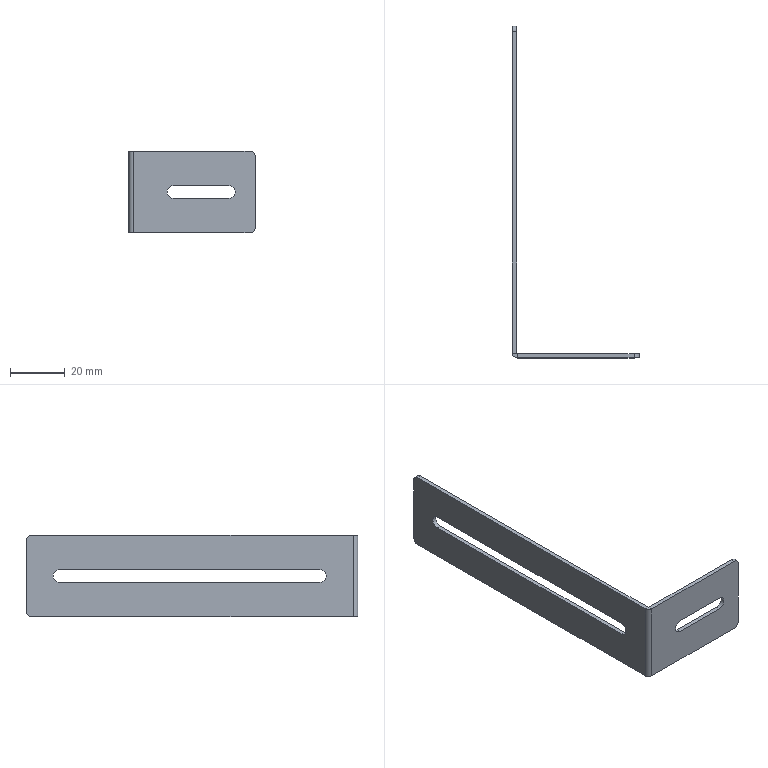Part | STEP file | FBDS-BJ-023 | 1 solid | 26 faces | box 46.5 x 121.5 x 30 mm | volume 6584 mm3 | plane 16 | cylinder 10 | commonest cylinder face diameters 4 x4 4.8 x4 0.4 x1 3.4 x1
STEP:
#1=CARTESIAN_POINT('',(0.2,0.,15.));
#2=VERTEX_POINT('',#1);
#3=CARTESIAN_POINT('',(0.2,-1.5,15.));
#4=VERTEX_POINT('',#3);
#5=CARTESIAN_POINT('',(0.2,0.,15.));
#6=DIRECTION('',(0.,-1.,0.));
#7=VECTOR('',#6,1000.);
#8=LINE('',#5,#7);
#9=EDGE_CURVE('',#2,#4,#8,.T.);
#10=ORIENTED_EDGE('',*,*,#9,.F.);
#11=CARTESIAN_POINT('',(0.,0.2,15.));
#12=VERTEX_POINT('',#11);
#13=CARTESIAN_POINT('',(0.2,0.2,15.));
#14=DIRECTION('',(0.,0.,1.));
#15=DIRECTION('',(-1.,0.,0.));
#16=AXIS2_PLACEMENT_3D('',#13,#14,#15);
#17=CIRCLE('',#16,0.2);
#18=EDGE_CURVE('',#12,#2,#17,.T.);
#19=ORIENTED_EDGE('',*,*,#18,.F.);
#20=CARTESIAN_POINT('',(-1.5,0.2,15.));
#21=VERTEX_POINT('',#20);
#22=CARTESIAN_POINT('',(-1.5,0.2,15.));
#23=DIRECTION('',(1.,0.,0.));
#24=VECTOR('',#23,1000.);
#25=LINE('',#22,#24);
#26=EDGE_CURVE('',#21,#12,#25,.T.);
#27=ORIENTED_EDGE('',*,*,#26,.F.);
#28=CARTESIAN_POINT('',(0.2,0.2,15.));
#29=DIRECTION('',(0.,0.,1.));
#30=DIRECTION('',(1.,0.,0.));
#31=AXIS2_PLACEMENT_3D('',#28,#29,#30);
#32=CIRCLE('',#31,1.7);
#33=EDGE_CURVE('',#21,#4,#32,.T.);
#34=ORIENTED_EDGE('',*,*,#33,.T.);
#35=EDGE_LOOP('',(#10,#19,#27,#34));
#36=FACE_OUTER_BOUND('',#35,.T.);
#37=CARTESIAN_POINT('',(0.2,0.,15.));
#38=DIRECTION('',(0.,0.,1.));
#39=DIRECTION('',(1.,0.,0.));
#40=AXIS2_PLACEMENT_3D('',#37,#38,#39);
#41=PLANE('',#40);
#42=ADVANCED_FACE('',(#36),#41,.T.);
#43=CARTESIAN_POINT('',(43.,-1.5,15.));
#44=VERTEX_POINT('',#43);
#45=CARTESIAN_POINT('',(0.,-1.5,15.));
#46=DIRECTION('',(1.,0.,0.));
#47=VECTOR('',#46,1000.);
#48=LINE('',#45,#47);
#49=EDGE_CURVE('',#4,#44,#48,.T.);
#50=ORIENTED_EDGE('',*,*,#49,.T.);
#51=CARTESIAN_POINT('',(43.,0.,15.));
#52=VERTEX_POINT('',#51);
#53=CARTESIAN_POINT('',(43.,0.2,15.));
#54=DIRECTION('',(0.,1.,0.));
#55=VECTOR('',#54,1000.);
#56=LINE('',#53,#55);
#57=EDGE_CURVE('',#44,#52,#56,.T.);
#58=ORIENTED_EDGE('',*,*,#57,.T.);
#59=CARTESIAN_POINT('',(0.,0.,15.));
#60=DIRECTION('',(1.,0.,0.));
#61=VECTOR('',#60,1000.);
#62=LINE('',#59,#61);
#63=EDGE_CURVE('',#2,#52,#62,.T.);
#64=ORIENTED_EDGE('',*,*,#63,.F.);
#65=ORIENTED_EDGE('',*,*,#9,.T.);
#66=EDGE_LOOP('',(#50,#58,#64,#65));
#67=FACE_OUTER_BOUND('',#66,.T.);
#68=CARTESIAN_POINT('',(-1.5,0.2,15.));
#69=DIRECTION('',(0.,0.,1.));
#70=DIRECTION('',(1.,0.,0.));
#71=AXIS2_PLACEMENT_3D('',#68,#69,#70);
#72=PLANE('',#71);
#73=ADVANCED_FACE('',(#67),#72,.T.);
#74=CARTESIAN_POINT('',(0.,0.2,-15.));
#75=VERTEX_POINT('',#74);
#76=CARTESIAN_POINT('',(-1.5,0.2,-15.));
#77=VERTEX_POINT('',#76);
#78=CARTESIAN_POINT('',(0.,0.2,-15.));
#79=DIRECTION('',(-1.,0.,0.));
#80=VECTOR('',#79,1000.);
#81=LINE('',#78,#80);
#82=EDGE_CURVE('',#75,#77,#81,.T.);
#83=ORIENTED_EDGE('',*,*,#82,.F.);
#84=CARTESIAN_POINT('',(0.2,0.,-15.));
#85=VERTEX_POINT('',#84);
#86=CARTESIAN_POINT('',(0.2,0.2,-15.));
#87=DIRECTION('',(0.,0.,1.));
#88=DIRECTION('',(-1.,0.,0.));
#89=AXIS2_PLACEMENT_3D('',#86,#87,#88);
#90=CIRCLE('',#89,0.2);
#91=EDGE_CURVE('',#75,#85,#90,.T.);
#92=ORIENTED_EDGE('',*,*,#91,.T.);
#93=CARTESIAN_POINT('',(0.2,-1.5,-15.));
#94=VERTEX_POINT('',#93);
#95=CARTESIAN_POINT('',(0.2,-1.5,-15.));
#96=DIRECTION('',(0.,1.,0.));
#97=VECTOR('',#96,1000.);
#98=LINE('',#95,#97);
#99=EDGE_CURVE('',#94,#85,#98,.T.);
#100=ORIENTED_EDGE('',*,*,#99,.F.);
#101=CARTESIAN_POINT('',(0.2,0.2,-15.));
#102=DIRECTION('',(0.,0.,1.));
#103=DIRECTION('',(1.,0.,0.));
#104=AXIS2_PLACEMENT_3D('',#101,#102,#103);
#105=CIRCLE('',#104,1.7);
#106=EDGE_CURVE('',#77,#94,#105,.T.);
#107=ORIENTED_EDGE('',*,*,#106,.F.);
#108=EDGE_LOOP('',(#83,#92,#100,#107));
#109=FACE_OUTER_BOUND('',#108,.T.);
#110=CARTESIAN_POINT('',(0.,0.2,-15.));
#111=DIRECTION('',(0.,0.,-1.));
#112=DIRECTION('',(-1.,0.,0.));
#113=AXIS2_PLACEMENT_3D('',#110,#111,#112);
#114=PLANE('',#113);
#115=ADVANCED_FACE('',(#109),#114,.T.);
#116=CARTESIAN_POINT('',(-1.5,118.,-15.));
#117=VERTEX_POINT('',#116);
#118=CARTESIAN_POINT('',(-1.5,120.,-15.));
#119=DIRECTION('',(0.,-1.,0.));
#120=VECTOR('',#119,1000.);
#121=LINE('',#118,#120);
#122=EDGE_CURVE('',#117,#77,#121,.T.);
#123=ORIENTED_EDGE('',*,*,#122,.F.);
#124=CARTESIAN_POINT('',(0.,118.,-15.));
#125=VERTEX_POINT('',#124);
#126=CARTESIAN_POINT('',(0.2,118.,-15.));
#127=DIRECTION('',(1.,0.,0.));
#128=VECTOR('',#127,1000.);
#129=LINE('',#126,#128);
#130=EDGE_CURVE('',#117,#125,#129,.T.);
#131=ORIENTED_EDGE('',*,*,#130,.T.);
#132=CARTESIAN_POINT('',(0.,120.,-15.));
#133=DIRECTION('',(0.,-1.,0.));
#134=VECTOR('',#133,1000.);
#135=LINE('',#132,#134);
#136=EDGE_CURVE('',#125,#75,#135,.T.);
#137=ORIENTED_EDGE('',*,*,#136,.T.);
#138=ORIENTED_EDGE('',*,*,#82,.T.);
#139=EDGE_LOOP('',(#123,#131,#137,#138));
#140=FACE_OUTER_BOUND('',#139,.T.);
#141=CARTESIAN_POINT('',(0.2,-1.5,-15.));
#142=DIRECTION('',(0.,0.,-1.));
#143=DIRECTION('',(-1.,0.,0.));
#144=AXIS2_PLACEMENT_3D('',#141,#142,#143);
#145=PLANE('',#144);
#146=ADVANCED_FACE('',(#140),#145,.T.);
#147=CARTESIAN_POINT('',(35.2,-1.5,-2.4));
#148=VERTEX_POINT('',#147);
#149=CARTESIAN_POINT('',(35.2,-1.5,2.4));
#150=VERTEX_POINT('',#149);
#151=CARTESIAN_POINT('',(35.2,-1.5,0.));
#152=DIRECTION('',(0.,-1.,0.));
#153=DIRECTION('',(0.,0.,-1.));
#154=AXIS2_PLACEMENT_3D('',#151,#152,#153);
#155=CIRCLE('',#154,2.4);
#156=EDGE_CURVE('',#148,#150,#155,.T.);
#157=ORIENTED_EDGE('',*,*,#156,.F.);
#158=CARTESIAN_POINT('',(15.,-1.5,-2.4));
#159=VERTEX_POINT('',#158);
#160=CARTESIAN_POINT('',(35.2,-1.5,-2.4));
#161=DIRECTION('',(-1.,0.,0.));
#162=VECTOR('',#161,1000.);
#163=LINE('',#160,#162);
#164=EDGE_CURVE('',#148,#159,#163,.T.);
#165=ORIENTED_EDGE('',*,*,#164,.T.);
#166=CARTESIAN_POINT('',(15.,-1.5,2.4));
#167=VERTEX_POINT('',#166);
#168=CARTESIAN_POINT('',(15.,-1.5,0.));
#169=DIRECTION('',(0.,-1.,0.));
#170=DIRECTION('',(0.,0.,-1.));
#171=AXIS2_PLACEMENT_3D('',#168,#169,#170);
#172=CIRCLE('',#171,2.4);
#173=EDGE_CURVE('',#167,#159,#172,.T.);
#174=ORIENTED_EDGE('',*,*,#173,.F.);
#175=CARTESIAN_POINT('',(35.2,-1.5,2.4));
#176=DIRECTION('',(-1.,0.,0.));
#177=VECTOR('',#176,1000.);
#178=LINE('',#175,#177);
#179=EDGE_CURVE('',#150,#167,#178,.T.);
#180=ORIENTED_EDGE('',*,*,#179,.F.);
#181=EDGE_LOOP('',(#157,#165,#174,#180));
#182=FACE_BOUND('',#181,.T.);
#183=CARTESIAN_POINT('',(43.,-1.5,-15.));
#184=VERTEX_POINT('',#183);
#185=CARTESIAN_POINT('',(0.,-1.5,-15.));
#186=DIRECTION('',(1.,0.,0.));
#187=VECTOR('',#186,1000.);
#188=LINE('',#185,#187);
#189=EDGE_CURVE('',#94,#184,#188,.T.);
#190=ORIENTED_EDGE('',*,*,#189,.T.);
#191=CARTESIAN_POINT('',(45.,-1.5,-13.));
#192=VERTEX_POINT('',#191);
#193=CARTESIAN_POINT('',(43.,-1.5,-13.));
#194=DIRECTION('',(0.,-1.,0.));
#195=DIRECTION('',(0.,0.,1.));
#196=AXIS2_PLACEMENT_3D('',#193,#194,#195);
#197=CIRCLE('',#196,2.);
#198=EDGE_CURVE('',#184,#192,#197,.T.);
#199=ORIENTED_EDGE('',*,*,#198,.T.);
#200=CARTESIAN_POINT('',(45.,-1.5,13.));
#201=VERTEX_POINT('',#200);
#202=CARTESIAN_POINT('',(45.,-1.5,15.));
#203=DIRECTION('',(0.,0.,-1.));
#204=VECTOR('',#203,1000.);
#205=LINE('',#202,#204);
#206=EDGE_CURVE('',#201,#192,#205,.T.);
#207=ORIENTED_EDGE('',*,*,#206,.F.);
#208=CARTESIAN_POINT('',(43.,-1.5,13.));
#209=DIRECTION('',(0.,-1.,0.));
#210=DIRECTION('',(0.,0.,1.));
#211=AXIS2_PLACEMENT_3D('',#208,#209,#210);
#212=CIRCLE('',#211,2.);
#213=EDGE_CURVE('',#201,#44,#212,.T.);
#214=ORIENTED_EDGE('',*,*,#213,.T.);
#215=ORIENTED_EDGE('',*,*,#49,.F.);
#216=CARTESIAN_POINT('',(0.2,-1.5,15.));
#217=DIRECTION('',(0.,0.,-1.));
#218=VECTOR('',#217,1000.);
#219=LINE('',#216,#218);
#220=EDGE_CURVE('',#4,#94,#219,.T.);
#221=ORIENTED_EDGE('',*,*,#220,.T.);
#222=EDGE_LOOP('',(#190,#199,#207,#214,#215,#221));
#223=FACE_OUTER_BOUND('',#222,.T.);
#224=CARTESIAN_POINT('',(0.,-1.5,15.));
#225=DIRECTION('',(0.,1.,0.));
#226=DIRECTION('',(0.,0.,1.));
#227=AXIS2_PLACEMENT_3D('',#224,#225,#226);
#228=PLANE('',#227);
#229=ADVANCED_FACE('',(#182,#223),#228,.F.);
#230=ORIENTED_EDGE('',*,*,#206,.T.);
#231=CARTESIAN_POINT('',(45.,0.,-13.));
#232=VERTEX_POINT('',#231);
#233=CARTESIAN_POINT('',(45.,0.,-13.));
#234=DIRECTION('',(0.,1.,0.));
#235=VECTOR('',#234,1000.);
#236=LINE('',#233,#235);
#237=EDGE_CURVE('',#192,#232,#236,.T.);
#238=ORIENTED_EDGE('',*,*,#237,.T.);
#239=CARTESIAN_POINT('',(45.,0.,13.));
#240=VERTEX_POINT('',#239);
#241=CARTESIAN_POINT('',(45.,0.,15.));
#242=DIRECTION('',(0.,0.,-1.));
#243=VECTOR('',#242,1000.);
#244=LINE('',#241,#243);
#245=EDGE_CURVE('',#240,#232,#244,.T.);
#246=ORIENTED_EDGE('',*,*,#245,.F.);
#247=CARTESIAN_POINT('',(45.,0.,13.));
#248=DIRECTION('',(0.,-1.,0.));
#249=VECTOR('',#248,1000.);
#250=LINE('',#247,#249);
#251=EDGE_CURVE('',#240,#201,#250,.T.);
#252=ORIENTED_EDGE('',*,*,#251,.T.);
#253=EDGE_LOOP('',(#230,#238,#246,#252));
#254=FACE_OUTER_BOUND('',#253,.T.);
#255=CARTESIAN_POINT('',(45.,0.,15.));
#256=DIRECTION('',(1.,0.,0.));
#257=DIRECTION('',(0.,0.,-1.));
#258=AXIS2_PLACEMENT_3D('',#255,#256,#257);
#259=PLANE('',#258);
#260=ADVANCED_FACE('',(#254),#259,.T.);
#261=CARTESIAN_POINT('',(15.,0.,2.4));
#262=VERTEX_POINT('',#261);
#263=CARTESIAN_POINT('',(15.,0.,-2.4));
#264=VERTEX_POINT('',#263);
#265=CARTESIAN_POINT('',(15.,0.,0.));
#266=DIRECTION('',(0.,-1.,0.));
#267=DIRECTION('',(0.,0.,-1.));
#268=AXIS2_PLACEMENT_3D('',#265,#266,#267);
#269=CIRCLE('',#268,2.4);
#270=EDGE_CURVE('',#262,#264,#269,.T.);
#271=ORIENTED_EDGE('',*,*,#270,.T.);
#272=CARTESIAN_POINT('',(35.2,0.,-2.4));
#273=VERTEX_POINT('',#272);
#274=CARTESIAN_POINT('',(35.2,0.,-2.4));
#275=DIRECTION('',(-1.,0.,0.));
#276=VECTOR('',#275,1000.);
#277=LINE('',#274,#276);
#278=EDGE_CURVE('',#273,#264,#277,.T.);
#279=ORIENTED_EDGE('',*,*,#278,.F.);
#280=CARTESIAN_POINT('',(35.2,0.,2.4));
#281=VERTEX_POINT('',#280);
#282=CARTESIAN_POINT('',(35.2,0.,0.));
#283=DIRECTION('',(0.,-1.,0.));
#284=DIRECTION('',(0.,0.,-1.));
#285=AXIS2_PLACEMENT_3D('',#282,#283,#284);
#286=CIRCLE('',#285,2.4);
#287=EDGE_CURVE('',#273,#281,#286,.T.);
#288=ORIENTED_EDGE('',*,*,#287,.T.);
#289=CARTESIAN_POINT('',(35.2,0.,2.4));
#290=DIRECTION('',(-1.,0.,0.));
#291=VECTOR('',#290,1000.);
#292=LINE('',#289,#291);
#293=EDGE_CURVE('',#281,#262,#292,.T.);
#294=ORIENTED_EDGE('',*,*,#293,.T.);
#295=EDGE_LOOP('',(#271,#279,#288,#294));
#296=FACE_BOUND('',#295,.T.);
#297=ORIENTED_EDGE('',*,*,#245,.T.);
#298=CARTESIAN_POINT('',(43.,0.,-15.));
#299=VERTEX_POINT('',#298);
#300=CARTESIAN_POINT('',(43.,0.,-13.));
#301=DIRECTION('',(0.,1.,0.));
#302=DIRECTION('',(0.,0.,1.));
#303=AXIS2_PLACEMENT_3D('',#300,#301,#302);
#304=CIRCLE('',#303,2.);
#305=EDGE_CURVE('',#232,#299,#304,.T.);
#306=ORIENTED_EDGE('',*,*,#305,.T.);
#307=CARTESIAN_POINT('',(0.,0.,-15.));
#308=DIRECTION('',(1.,0.,0.));
#309=VECTOR('',#308,1000.);
#310=LINE('',#307,#309);
#311=EDGE_CURVE('',#85,#299,#310,.T.);
#312=ORIENTED_EDGE('',*,*,#311,.F.);
#313=CARTESIAN_POINT('',(0.2,0.,15.));
#314=DIRECTION('',(0.,0.,-1.));
#315=VECTOR('',#314,1000.);
#316=LINE('',#313,#315);
#317=EDGE_CURVE('',#2,#85,#316,.T.);
#318=ORIENTED_EDGE('',*,*,#317,.F.);
#319=ORIENTED_EDGE('',*,*,#63,.T.);
#320=CARTESIAN_POINT('',(43.,0.,13.));
#321=DIRECTION('',(0.,1.,0.));
#322=DIRECTION('',(0.,0.,1.));
#323=AXIS2_PLACEMENT_3D('',#320,#321,#322);
#324=CIRCLE('',#323,2.);
#325=EDGE_CURVE('',#52,#240,#324,.T.);
#326=ORIENTED_EDGE('',*,*,#325,.T.);
#327=EDGE_LOOP('',(#297,#306,#312,#318,#319,#326));
#328=FACE_OUTER_BOUND('',#327,.T.);
#329=CARTESIAN_POINT('',(0.,0.,15.));
#330=DIRECTION('',(0.,1.,0.));
#331=DIRECTION('',(0.,0.,1.));
#332=AXIS2_PLACEMENT_3D('',#329,#330,#331);
#333=PLANE('',#332);
#334=ADVANCED_FACE('',(#296,#328),#333,.T.);
#335=ORIENTED_EDGE('',*,*,#91,.F.);
#336=CARTESIAN_POINT('',(0.,0.2,15.));
#337=DIRECTION('',(0.,0.,-1.));
#338=VECTOR('',#337,1000.);
#339=LINE('',#336,#338);
#340=EDGE_CURVE('',#12,#75,#339,.T.);
#341=ORIENTED_EDGE('',*,*,#340,.F.);
#342=ORIENTED_EDGE('',*,*,#18,.T.);
#343=ORIENTED_EDGE('',*,*,#317,.T.);
#344=EDGE_LOOP('',(#335,#341,#342,#343));
#345=FACE_OUTER_BOUND('',#344,.T.);
#346=CARTESIAN_POINT('',(0.2,0.2,15.));
#347=DIRECTION('',(0.,0.,-1.));
#348=DIRECTION('',(-1.,0.,0.));
#349=AXIS2_PLACEMENT_3D('',#346,#347,#348);
#350=CYLINDRICAL_SURFACE('',#349,0.2);
#351=ADVANCED_FACE('',(#345),#350,.F.);
#352=CARTESIAN_POINT('',(0.,12.5,2.4));
#353=VERTEX_POINT('',#352);
#354=CARTESIAN_POINT('',(0.,107.7,2.4));
#355=VERTEX_POINT('',#354);
#356=CARTESIAN_POINT('',(0.,12.5,2.4));
#357=DIRECTION('',(0.,1.,0.));
#358=VECTOR('',#357,1000.);
#359=LINE('',#356,#358);
#360=EDGE_CURVE('',#353,#355,#359,.T.);
#361=ORIENTED_EDGE('',*,*,#360,.T.);
#362=CARTESIAN_POINT('',(0.,107.7,-2.4));
#363=VERTEX_POINT('',#362);
#364=CARTESIAN_POINT('',(0.,107.7,0.));
#365=DIRECTION('',(-1.,0.,0.));
#366=DIRECTION('',(0.,0.,1.));
#367=AXIS2_PLACEMENT_3D('',#364,#365,#366);
#368=CIRCLE('',#367,2.4);
#369=EDGE_CURVE('',#355,#363,#368,.T.);
#370=ORIENTED_EDGE('',*,*,#369,.T.);
#371=CARTESIAN_POINT('',(0.,12.5,-2.4));
#372=VERTEX_POINT('',#371);
#373=CARTESIAN_POINT('',(0.,12.5,-2.4));
#374=DIRECTION('',(0.,1.,0.));
#375=VECTOR('',#374,1000.);
#376=LINE('',#373,#375);
#377=EDGE_CURVE('',#372,#363,#376,.T.);
#378=ORIENTED_EDGE('',*,*,#377,.F.);
#379=CARTESIAN_POINT('',(0.,12.5,0.));
#380=DIRECTION('',(-1.,0.,0.));
#381=DIRECTION('',(0.,0.,1.));
#382=AXIS2_PLACEMENT_3D('',#379,#380,#381);
#383=CIRCLE('',#382,2.4);
#384=EDGE_CURVE('',#372,#353,#383,.T.);
#385=ORIENTED_EDGE('',*,*,#384,.T.);
#386=EDGE_LOOP('',(#361,#370,#378,#385));
#387=FACE_BOUND('',#386,.T.);
#388=ORIENTED_EDGE('',*,*,#136,.F.);
#389=CARTESIAN_POINT('',(0.,120.,-13.));
#390=VERTEX_POINT('',#389);
#391=CARTESIAN_POINT('',(0.,118.,-13.));
#392=DIRECTION('',(1.,0.,0.));
#393=DIRECTION('',(0.,1.,0.));
#394=AXIS2_PLACEMENT_3D('',#391,#392,#393);
#395=CIRCLE('',#394,2.);
#396=EDGE_CURVE('',#125,#390,#395,.T.);
#397=ORIENTED_EDGE('',*,*,#396,.T.);
#398=CARTESIAN_POINT('',(0.,120.,13.));
#399=VERTEX_POINT('',#398);
#400=CARTESIAN_POINT('',(0.,120.,15.));
#401=DIRECTION('',(0.,0.,-1.));
#402=VECTOR('',#401,1000.);
#403=LINE('',#400,#402);
#404=EDGE_CURVE('',#399,#390,#403,.T.);
#405=ORIENTED_EDGE('',*,*,#404,.F.);
#406=CARTESIAN_POINT('',(0.,118.,15.));
#407=VERTEX_POINT('',#406);
#408=CARTESIAN_POINT('',(0.,118.,13.));
#409=DIRECTION('',(1.,0.,0.));
#410=DIRECTION('',(0.,1.,0.));
#411=AXIS2_PLACEMENT_3D('',#408,#409,#410);
#412=CIRCLE('',#411,2.);
#413=EDGE_CURVE('',#399,#407,#412,.T.);
#414=ORIENTED_EDGE('',*,*,#413,.T.);
#415=CARTESIAN_POINT('',(0.,120.,15.));
#416=DIRECTION('',(0.,-1.,0.));
#417=VECTOR('',#416,1000.);
#418=LINE('',#415,#417);
#419=EDGE_CURVE('',#407,#12,#418,.T.);
#420=ORIENTED_EDGE('',*,*,#419,.T.);
#421=ORIENTED_EDGE('',*,*,#340,.T.);
#422=EDGE_LOOP('',(#388,#397,#405,#414,#420,#421));
#423=FACE_OUTER_BOUND('',#422,.T.);
#424=CARTESIAN_POINT('',(0.,120.,15.));
#425=DIRECTION('',(1.,0.,0.));
#426=DIRECTION('',(0.,1.,0.));
#427=AXIS2_PLACEMENT_3D('',#424,#425,#426);
#428=PLANE('',#427);
#429=ADVANCED_FACE('',(#387,#423),#428,.T.);
#430=ORIENTED_EDGE('',*,*,#404,.T.);
#431=CARTESIAN_POINT('',(-1.5,120.,-13.));
#432=VERTEX_POINT('',#431);
#433=CARTESIAN_POINT('',(-1.5,120.,-13.));
#434=DIRECTION('',(-1.,0.,0.));
#435=VECTOR('',#434,1000.);
#436=LINE('',#433,#435);
#437=EDGE_CURVE('',#390,#432,#436,.T.);
#438=ORIENTED_EDGE('',*,*,#437,.T.);
#439=CARTESIAN_POINT('',(-1.5,120.,13.));
#440=VERTEX_POINT('',#439);
#441=CARTESIAN_POINT('',(-1.5,120.,15.));
#442=DIRECTION('',(0.,0.,-1.));
#443=VECTOR('',#442,1000.);
#444=LINE('',#441,#443);
#445=EDGE_CURVE('',#440,#432,#444,.T.);
#446=ORIENTED_EDGE('',*,*,#445,.F.);
#447=CARTESIAN_POINT('',(0.,120.,13.));
#448=DIRECTION('',(1.,0.,0.));
#449=VECTOR('',#448,1000.);
#450=LINE('',#447,#449);
#451=EDGE_CURVE('',#440,#399,#450,.T.);
#452=ORIENTED_EDGE('',*,*,#451,.T.);
#453=EDGE_LOOP('',(#430,#438,#446,#452));
#454=FACE_OUTER_BOUND('',#453,.T.);
#455=CARTESIAN_POINT('',(-1.5,120.,15.));
#456=DIRECTION('',(0.,1.,0.));
#457=DIRECTION('',(0.,0.,1.));
#458=AXIS2_PLACEMENT_3D('',#455,#456,#457);
#459=PLANE('',#458);
#460=ADVANCED_FACE('',(#454),#459,.T.);
#461=CARTESIAN_POINT('',(-1.5,12.5,-2.4));
#462=VERTEX_POINT('',#461);
#463=CARTESIAN_POINT('',(-1.5,107.7,-2.4));
#464=VERTEX_POINT('',#463);
#465=CARTESIAN_POINT('',(-1.5,12.5,-2.4));
#466=DIRECTION('',(0.,1.,0.));
#467=VECTOR('',#466,1000.);
#468=LINE('',#465,#467);
#469=EDGE_CURVE('',#462,#464,#468,.T.);
#470=ORIENTED_EDGE('',*,*,#469,.T.);
#471=CARTESIAN_POINT('',(-1.5,107.7,2.4));
#472=VERTEX_POINT('',#471);
#473=CARTESIAN_POINT('',(-1.5,107.7,0.));
#474=DIRECTION('',(-1.,0.,0.));
#475=DIRECTION('',(0.,0.,1.));
#476=AXIS2_PLACEMENT_3D('',#473,#474,#475);
#477=CIRCLE('',#476,2.4);
#478=EDGE_CURVE('',#472,#464,#477,.T.);
#479=ORIENTED_EDGE('',*,*,#478,.F.);
#480=CARTESIAN_POINT('',(-1.5,12.5,2.4));
#481=VERTEX_POINT('',#480);
#482=CARTESIAN_POINT('',(-1.5,12.5,2.4));
#483=DIRECTION('',(0.,1.,0.));
#484=VECTOR('',#483,1000.);
#485=LINE('',#482,#484);
#486=EDGE_CURVE('',#481,#472,#485,.T.);
#487=ORIENTED_EDGE('',*,*,#486,.F.);
#488=CARTESIAN_POINT('',(-1.5,12.5,0.));
#489=DIRECTION('',(-1.,0.,0.));
#490=DIRECTION('',(0.,0.,1.));
#491=AXIS2_PLACEMENT_3D('',#488,#489,#490);
#492=CIRCLE('',#491,2.4);
#493=EDGE_CURVE('',#462,#481,#492,.T.);
#494=ORIENTED_EDGE('',*,*,#493,.F.);
#495=EDGE_LOOP('',(#470,#479,#487,#494));
#496=FACE_BOUND('',#495,.T.);
#497=ORIENTED_EDGE('',*,*,#445,.T.);
#498=CARTESIAN_POINT('',(-1.5,118.,-13.));
#499=DIRECTION('',(-1.,0.,0.));
#500=DIRECTION('',(0.,1.,0.));
#501=AXIS2_PLACEMENT_3D('',#498,#499,#500);
#502=CIRCLE('',#501,2.);
#503=EDGE_CURVE('',#432,#117,#502,.T.);
#504=ORIENTED_EDGE('',*,*,#503,.T.);
#505=ORIENTED_EDGE('',*,*,#122,.T.);
#506=CARTESIAN_POINT('',(-1.5,0.2,15.));
#507=DIRECTION('',(0.,0.,-1.));
#508=VECTOR('',#507,1000.);
#509=LINE('',#506,#508);
#510=EDGE_CURVE('',#21,#77,#509,.T.);
#511=ORIENTED_EDGE('',*,*,#510,.F.);
#512=CARTESIAN_POINT('',(-1.5,118.,15.));
#513=VERTEX_POINT('',#512);
#514=CARTESIAN_POINT('',(-1.5,120.,15.));
#515=DIRECTION('',(0.,-1.,0.));
#516=VECTOR('',#515,1000.);
#517=LINE('',#514,#516);
#518=EDGE_CURVE('',#513,#21,#517,.T.);
#519=ORIENTED_EDGE('',*,*,#518,.F.);
#520=CARTESIAN_POINT('',(-1.5,118.,13.));
#521=DIRECTION('',(-1.,0.,0.));
#522=DIRECTION('',(0.,1.,0.));
#523=AXIS2_PLACEMENT_3D('',#520,#521,#522);
#524=CIRCLE('',#523,2.);
#525=EDGE_CURVE('',#513,#440,#524,.T.);
#526=ORIENTED_EDGE('',*,*,#525,.T.);
#527=EDGE_LOOP('',(#497,#504,#505,#511,#519,#526));
#528=FACE_OUTER_BOUND('',#527,.T.);
#529=CARTESIAN_POINT('',(-1.5,120.,15.));
#530=DIRECTION('',(1.,0.,0.));
#531=DIRECTION('',(0.,1.,0.));
#532=AXIS2_PLACEMENT_3D('',#529,#530,#531);
#533=PLANE('',#532);
#534=ADVANCED_FACE('',(#496,#528),#533,.F.);
#535=ORIENTED_EDGE('',*,*,#106,.T.);
#536=ORIENTED_EDGE('',*,*,#220,.F.);
#537=ORIENTED_EDGE('',*,*,#33,.F.);
#538=ORIENTED_EDGE('',*,*,#510,.T.);
#539=EDGE_LOOP('',(#535,#536,#537,#538));
#540=FACE_OUTER_BOUND('',#539,.T.);
#541=CARTESIAN_POINT('',(0.2,0.2,15.));
#542=DIRECTION('',(0.,0.,-1.));
#543=DIRECTION('',(-1.,0.,0.));
#544=AXIS2_PLACEMENT_3D('',#541,#542,#543);
#545=CYLINDRICAL_SURFACE('',#544,1.7);
#546=ADVANCED_FACE('',(#540),#545,.T.);
#547=ORIENTED_EDGE('',*,*,#419,.F.);
#548=CARTESIAN_POINT('',(-1.5,118.,15.));
#549=DIRECTION('',(-1.,0.,0.));
#550=VECTOR('',#549,1000.);
#551=LINE('',#548,#550);
#552=EDGE_CURVE('',#407,#513,#551,.T.);
#553=ORIENTED_EDGE('',*,*,#552,.T.);
#554=ORIENTED_EDGE('',*,*,#518,.T.);
#555=ORIENTED_EDGE('',*,*,#26,.T.);
#556=EDGE_LOOP('',(#547,#553,#554,#555));
#557=FACE_OUTER_BOUND('',#556,.T.);
#558=CARTESIAN_POINT('',(0.2,0.2,15.));
#559=DIRECTION('',(0.,0.,-1.));
#560=DIRECTION('',(-1.,0.,0.));
#561=AXIS2_PLACEMENT_3D('',#558,#559,#560);
#562=PLANE('',#561);
#563=ADVANCED_FACE('',(#557),#562,.F.);
#564=ORIENTED_EDGE('',*,*,#311,.T.);
#565=CARTESIAN_POINT('',(43.,0.2,-15.));
#566=DIRECTION('',(0.,-1.,0.));
#567=VECTOR('',#566,1000.);
#568=LINE('',#565,#567);
#569=EDGE_CURVE('',#299,#184,#568,.T.);
#570=ORIENTED_EDGE('',*,*,#569,.T.);
#571=ORIENTED_EDGE('',*,*,#189,.F.);
#572=ORIENTED_EDGE('',*,*,#99,.T.);
#573=EDGE_LOOP('',(#564,#570,#571,#572));
#574=FACE_OUTER_BOUND('',#573,.T.);
#575=CARTESIAN_POINT('',(0.2,0.2,-15.));
#576=DIRECTION('',(0.,0.,-1.));
#577=DIRECTION('',(-1.,0.,0.));
#578=AXIS2_PLACEMENT_3D('',#575,#576,#577);
#579=PLANE('',#578);
#580=ADVANCED_FACE('',(#574),#579,.T.);
#581=ORIENTED_EDGE('',*,*,#369,.F.);
#582=CARTESIAN_POINT('',(-1.5,107.7,2.4));
#583=DIRECTION('',(1.,0.,0.));
#584=VECTOR('',#583,1000.);
#585=LINE('',#582,#584);
#586=EDGE_CURVE('',#472,#355,#585,.T.);
#587=ORIENTED_EDGE('',*,*,#586,.F.);
#588=ORIENTED_EDGE('',*,*,#478,.T.);
#589=CARTESIAN_POINT('',(-1.5,107.7,-2.4));
#590=DIRECTION('',(-1.,0.,0.));
#591=VECTOR('',#590,1000.);
#592=LINE('',#589,#591);
#593=EDGE_CURVE('',#363,#464,#592,.T.);
#594=ORIENTED_EDGE('',*,*,#593,.F.);
#595=EDGE_LOOP('',(#581,#587,#588,#594));
#596=FACE_OUTER_BOUND('',#595,.T.);
#597=CARTESIAN_POINT('',(-1.5,107.7,0.));
#598=DIRECTION('',(-1.,0.,0.));
#599=DIRECTION('',(0.,0.,1.));
#600=AXIS2_PLACEMENT_3D('',#597,#598,#599);
#601=CYLINDRICAL_SURFACE('',#600,2.4);
#602=ADVANCED_FACE('',(#596),#601,.F.);
#603=ORIENTED_EDGE('',*,*,#493,.T.);
#604=CARTESIAN_POINT('',(-1.5,12.5,2.4));
#605=DIRECTION('',(-1.,0.,0.));
#606=VECTOR('',#605,1000.);
#607=LINE('',#604,#606);
#608=EDGE_CURVE('',#353,#481,#607,.T.);
#609=ORIENTED_EDGE('',*,*,#608,.F.);
#610=ORIENTED_EDGE('',*,*,#384,.F.);
#611=CARTESIAN_POINT('',(-1.5,12.5,-2.4));
#612=DIRECTION('',(1.,0.,0.));
#613=VECTOR('',#612,1000.);
#614=LINE('',#611,#613);
#615=EDGE_CURVE('',#462,#372,#614,.T.);
#616=ORIENTED_EDGE('',*,*,#615,.F.);
#617=EDGE_LOOP('',(#603,#609,#610,#616));
#618=FACE_OUTER_BOUND('',#617,.T.);
#619=CARTESIAN_POINT('',(-1.5,12.5,0.));
#620=DIRECTION('',(-1.,0.,0.));
#621=DIRECTION('',(0.,0.,1.));
#622=AXIS2_PLACEMENT_3D('',#619,#620,#621);
#623=CYLINDRICAL_SURFACE('',#622,2.4);
#624=ADVANCED_FACE('',(#618),#623,.F.);
#625=ORIENTED_EDGE('',*,*,#593,.T.);
#626=ORIENTED_EDGE('',*,*,#469,.F.);
#627=ORIENTED_EDGE('',*,*,#615,.T.);
#628=ORIENTED_EDGE('',*,*,#377,.T.);
#629=EDGE_LOOP('',(#625,#626,#627,#628));
#630=FACE_OUTER_BOUND('',#629,.T.);
#631=CARTESIAN_POINT('',(-1.5,12.5,-2.4));
#632=DIRECTION('',(0.,0.,-1.));
#633=DIRECTION('',(-1.,0.,0.));
#634=AXIS2_PLACEMENT_3D('',#631,#632,#633);
#635=PLANE('',#634);
#636=ADVANCED_FACE('',(#630),#635,.F.);
#637=ORIENTED_EDGE('',*,*,#586,.T.);
#638=ORIENTED_EDGE('',*,*,#360,.F.);
#639=ORIENTED_EDGE('',*,*,#608,.T.);
#640=ORIENTED_EDGE('',*,*,#486,.T.);
#641=EDGE_LOOP('',(#637,#638,#639,#640));
#642=FACE_OUTER_BOUND('',#641,.T.);
#643=CARTESIAN_POINT('',(-1.5,12.5,2.4));
#644=DIRECTION('',(0.,0.,1.));
#645=DIRECTION('',(1.,0.,0.));
#646=AXIS2_PLACEMENT_3D('',#643,#644,#645);
#647=PLANE('',#646);
#648=ADVANCED_FACE('',(#642),#647,.F.);
#649=ORIENTED_EDGE('',*,*,#173,.T.);
#650=CARTESIAN_POINT('',(15.,-1.5,-2.4));
#651=DIRECTION('',(0.,-1.,0.));
#652=VECTOR('',#651,1000.);
#653=LINE('',#650,#652);
#654=EDGE_CURVE('',#264,#159,#653,.T.);
#655=ORIENTED_EDGE('',*,*,#654,.F.);
#656=ORIENTED_EDGE('',*,*,#270,.F.);
#657=CARTESIAN_POINT('',(15.,-1.5,2.4));
#658=DIRECTION('',(0.,1.,0.));
#659=VECTOR('',#658,1000.);
#660=LINE('',#657,#659);
#661=EDGE_CURVE('',#167,#262,#660,.T.);
#662=ORIENTED_EDGE('',*,*,#661,.F.);
#663=EDGE_LOOP('',(#649,#655,#656,#662));
#664=FACE_OUTER_BOUND('',#663,.T.);
#665=CARTESIAN_POINT('',(15.,-1.5,0.));
#666=DIRECTION('',(0.,-1.,0.));
#667=DIRECTION('',(0.,0.,-1.));
#668=AXIS2_PLACEMENT_3D('',#665,#666,#667);
#669=CYLINDRICAL_SURFACE('',#668,2.4);
#670=ADVANCED_FACE('',(#664),#669,.F.);
#671=ORIENTED_EDGE('',*,*,#156,.T.);
#672=CARTESIAN_POINT('',(35.2,-1.5,2.4));
#673=DIRECTION('',(0.,-1.,0.));
#674=VECTOR('',#673,1000.);
#675=LINE('',#672,#674);
#676=EDGE_CURVE('',#281,#150,#675,.T.);
#677=ORIENTED_EDGE('',*,*,#676,.F.);
#678=ORIENTED_EDGE('',*,*,#287,.F.);
#679=CARTESIAN_POINT('',(35.2,-1.5,-2.4));
#680=DIRECTION('',(0.,1.,0.));
#681=VECTOR('',#680,1000.);
#682=LINE('',#679,#681);
#683=EDGE_CURVE('',#148,#273,#682,.T.);
#684=ORIENTED_EDGE('',*,*,#683,.F.);
#685=EDGE_LOOP('',(#671,#677,#678,#684));
#686=FACE_OUTER_BOUND('',#685,.T.);
#687=CARTESIAN_POINT('',(35.2,-1.5,0.));
#688=DIRECTION('',(0.,-1.,0.));
#689=DIRECTION('',(0.,0.,-1.));
#690=AXIS2_PLACEMENT_3D('',#687,#688,#689);
#691=CYLINDRICAL_SURFACE('',#690,2.4);
#692=ADVANCED_FACE('',(#686),#691,.F.);
#693=ORIENTED_EDGE('',*,*,#654,.T.);
#694=ORIENTED_EDGE('',*,*,#164,.F.);
#695=ORIENTED_EDGE('',*,*,#683,.T.);
#696=ORIENTED_EDGE('',*,*,#278,.T.);
#697=EDGE_LOOP('',(#693,#694,#695,#696));
#698=FACE_OUTER_BOUND('',#697,.T.);
#699=CARTESIAN_POINT('',(35.2,-1.5,-2.4));
#700=DIRECTION('',(0.,0.,-1.));
#701=DIRECTION('',(-1.,0.,0.));
#702=AXIS2_PLACEMENT_3D('',#699,#700,#701);
#703=PLANE('',#702);
#704=ADVANCED_FACE('',(#698),#703,.F.);
#705=ORIENTED_EDGE('',*,*,#661,.T.);
#706=ORIENTED_EDGE('',*,*,#293,.F.);
#707=ORIENTED_EDGE('',*,*,#676,.T.);
#708=ORIENTED_EDGE('',*,*,#179,.T.);
#709=EDGE_LOOP('',(#705,#706,#707,#708));
#710=FACE_OUTER_BOUND('',#709,.T.);
#711=CARTESIAN_POINT('',(35.2,-1.5,2.4));
#712=DIRECTION('',(0.,0.,1.));
#713=DIRECTION('',(1.,0.,0.));
#714=AXIS2_PLACEMENT_3D('',#711,#712,#713);
#715=PLANE('',#714);
#716=ADVANCED_FACE('',(#710),#715,.F.);
#717=ORIENTED_EDGE('',*,*,#305,.F.);
#718=ORIENTED_EDGE('',*,*,#237,.F.);
#719=ORIENTED_EDGE('',*,*,#198,.F.);
#720=ORIENTED_EDGE('',*,*,#569,.F.);
#721=EDGE_LOOP('',(#717,#718,#719,#720));
#722=FACE_OUTER_BOUND('',#721,.T.);
#723=CARTESIAN_POINT('',(43.,0.2,-13.));
#724=DIRECTION('',(0.,-1.,0.));
#725=DIRECTION('',(0.,0.,-1.));
#726=AXIS2_PLACEMENT_3D('',#723,#724,#725);
#727=CYLINDRICAL_SURFACE('',#726,2.);
#728=ADVANCED_FACE('',(#722),#727,.T.);
#729=ORIENTED_EDGE('',*,*,#325,.F.);
#730=ORIENTED_EDGE('',*,*,#57,.F.);
#731=ORIENTED_EDGE('',*,*,#213,.F.);
#732=ORIENTED_EDGE('',*,*,#251,.F.);
#733=EDGE_LOOP('',(#729,#730,#731,#732));
#734=FACE_OUTER_BOUND('',#733,.T.);
#735=CARTESIAN_POINT('',(43.,0.,13.));
#736=DIRECTION('',(0.,-1.,0.));
#737=DIRECTION('',(0.,0.,-1.));
#738=AXIS2_PLACEMENT_3D('',#735,#736,#737);
#739=CYLINDRICAL_SURFACE('',#738,2.);
#740=ADVANCED_FACE('',(#734),#739,.T.);
#741=ORIENTED_EDGE('',*,*,#503,.F.);
#742=ORIENTED_EDGE('',*,*,#437,.F.);
#743=ORIENTED_EDGE('',*,*,#396,.F.);
#744=ORIENTED_EDGE('',*,*,#130,.F.);
#745=EDGE_LOOP('',(#741,#742,#743,#744));
#746=FACE_OUTER_BOUND('',#745,.T.);
#747=CARTESIAN_POINT('',(0.2,118.,-13.));
#748=DIRECTION('',(1.,0.,0.));
#749=DIRECTION('',(0.,0.,-1.));
#750=AXIS2_PLACEMENT_3D('',#747,#748,#749);
#751=CYLINDRICAL_SURFACE('',#750,2.);
#752=ADVANCED_FACE('',(#746),#751,.T.);
#753=ORIENTED_EDGE('',*,*,#525,.F.);
#754=ORIENTED_EDGE('',*,*,#552,.F.);
#755=ORIENTED_EDGE('',*,*,#413,.F.);
#756=ORIENTED_EDGE('',*,*,#451,.F.);
#757=EDGE_LOOP('',(#753,#754,#755,#756));
#758=FACE_OUTER_BOUND('',#757,.T.);
#759=CARTESIAN_POINT('',(-1.5,118.,13.));
#760=DIRECTION('',(-1.,0.,0.));
#761=DIRECTION('',(0.,0.,1.));
#762=AXIS2_PLACEMENT_3D('',#759,#760,#761);
#763=CYLINDRICAL_SURFACE('',#762,2.);
#764=ADVANCED_FACE('',(#758),#763,.T.);
#765=CLOSED_SHELL('',(#42,#73,#115,#146,#229,#260,#334,#351,#429,#460,#534,#546,#563,#580,#602,#624,#636,#648,#670,#692,#704,#716,#728,#740,#752,#764));
#766=MANIFOLD_SOLID_BREP('',#765);
#767=CARTESIAN_POINT('',(0.,0.,0.));
#768=DIRECTION('',(0.,0.,1.));
#769=DIRECTION('',(1.,0.,0.));
#770=AXIS2_PLACEMENT_3D('',#767,#768,#769);
#771=(LENGTH_UNIT()NAMED_UNIT(*)SI_UNIT(.MILLI.,.METRE.));
#772=UNCERTAINTY_MEASURE_WITH_UNIT(LENGTH_MEASURE(0.00001),#771,'','');
#773=(NAMED_UNIT(*)PLANE_ANGLE_UNIT()SI_UNIT($,.RADIAN.));
#774=(NAMED_UNIT(*)SI_UNIT($,.STERADIAN.)SOLID_ANGLE_UNIT());
#775=(GEOMETRIC_REPRESENTATION_CONTEXT(3)GLOBAL_UNCERTAINTY_ASSIGNED_CONTEXT((#772))GLOBAL_UNIT_ASSIGNED_CONTEXT((#771,#773,#774))REPRESENTATION_CONTEXT('',''));
#776=ADVANCED_BREP_SHAPE_REPRESENTATION('',(#766,#770),#775);